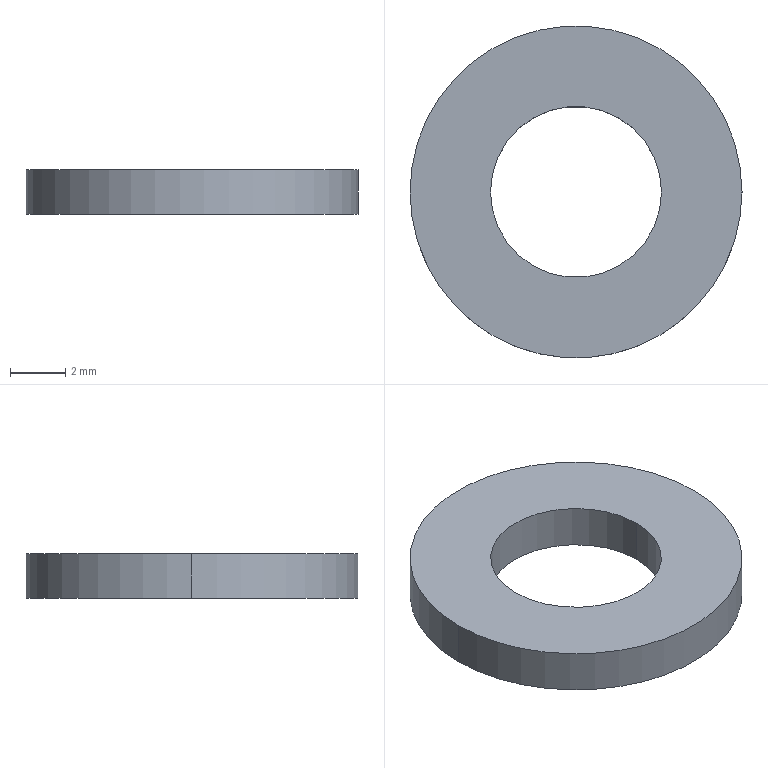Part | SolidWorks | features Extrusion 1 | 1 solid | 6 faces | box 12 x 12 x 1.6 mm | volume 132.962 mm3 | cylinder 4 | plane 2 | commonest cylinder face diameters 6.18 x2 12 x2
STEP:
#1=CARTESIAN_POINT('',(-3.09,0.,-1.6));
#2=VERTEX_POINT('',#1);
#3=CARTESIAN_POINT('',(3.09,0.,-1.6));
#4=VERTEX_POINT('',#3);
#5=CARTESIAN_POINT('',(0.,0.,-1.6));
#6=DIRECTION('',(0.,0.,1.));
#7=DIRECTION('',(1.,0.,0.));
#8=AXIS2_PLACEMENT_3D('',#5,#6,#7);
#9=CIRCLE('',#8,3.09);
#10=EDGE_CURVE('',#2,#4,#9,.T.);
#11=ORIENTED_EDGE('',*,*,#10,.F.);
#12=CARTESIAN_POINT('',(-3.09,0.,0.));
#13=VERTEX_POINT('',#12);
#14=CARTESIAN_POINT('',(-3.09,0.,-1.6));
#15=DIRECTION('',(0.,0.,1.));
#16=VECTOR('',#15,1000.);
#17=LINE('',#14,#16);
#18=EDGE_CURVE('',#2,#13,#17,.T.);
#19=ORIENTED_EDGE('',*,*,#18,.T.);
#20=CARTESIAN_POINT('',(3.09,0.,0.));
#21=VERTEX_POINT('',#20);
#22=CARTESIAN_POINT('',(0.,0.,0.));
#23=DIRECTION('',(0.,0.,1.));
#24=DIRECTION('',(1.,0.,0.));
#25=AXIS2_PLACEMENT_3D('',#22,#23,#24);
#26=CIRCLE('',#25,3.09);
#27=EDGE_CURVE('',#13,#21,#26,.T.);
#28=ORIENTED_EDGE('',*,*,#27,.T.);
#29=CARTESIAN_POINT('',(3.09,0.,-1.6));
#30=DIRECTION('',(0.,0.,1.));
#31=VECTOR('',#30,1000.);
#32=LINE('',#29,#31);
#33=EDGE_CURVE('',#4,#21,#32,.T.);
#34=ORIENTED_EDGE('',*,*,#33,.F.);
#35=EDGE_LOOP('',(#11,#19,#28,#34));
#36=FACE_OUTER_BOUND('',#35,.T.);
#37=CARTESIAN_POINT('',(0.,0.,-1.6));
#38=DIRECTION('',(0.,0.,1.));
#39=DIRECTION('',(1.,0.,0.));
#40=AXIS2_PLACEMENT_3D('',#37,#38,#39);
#41=CYLINDRICAL_SURFACE('',#40,3.09);
#42=ADVANCED_FACE('',(#36),#41,.F.);
#43=CARTESIAN_POINT('',(6.,0.,-1.6));
#44=VERTEX_POINT('',#43);
#45=CARTESIAN_POINT('',(-6.,0.,-1.6));
#46=VERTEX_POINT('',#45);
#47=CARTESIAN_POINT('',(0.,0.,-1.6));
#48=DIRECTION('',(0.,0.,1.));
#49=DIRECTION('',(1.,0.,0.));
#50=AXIS2_PLACEMENT_3D('',#47,#48,#49);
#51=CIRCLE('',#50,6.);
#52=EDGE_CURVE('',#44,#46,#51,.T.);
#53=ORIENTED_EDGE('',*,*,#52,.T.);
#54=CARTESIAN_POINT('',(-6.,0.,0.));
#55=VERTEX_POINT('',#54);
#56=CARTESIAN_POINT('',(-6.,0.,-1.6));
#57=DIRECTION('',(0.,0.,1.));
#58=VECTOR('',#57,1000.);
#59=LINE('',#56,#58);
#60=EDGE_CURVE('',#46,#55,#59,.T.);
#61=ORIENTED_EDGE('',*,*,#60,.T.);
#62=CARTESIAN_POINT('',(6.,0.,0.));
#63=VERTEX_POINT('',#62);
#64=CARTESIAN_POINT('',(0.,0.,0.));
#65=DIRECTION('',(0.,0.,1.));
#66=DIRECTION('',(1.,0.,0.));
#67=AXIS2_PLACEMENT_3D('',#64,#65,#66);
#68=CIRCLE('',#67,6.);
#69=EDGE_CURVE('',#63,#55,#68,.T.);
#70=ORIENTED_EDGE('',*,*,#69,.F.);
#71=CARTESIAN_POINT('',(6.,0.,-1.6));
#72=DIRECTION('',(0.,0.,1.));
#73=VECTOR('',#72,1000.);
#74=LINE('',#71,#73);
#75=EDGE_CURVE('',#44,#63,#74,.T.);
#76=ORIENTED_EDGE('',*,*,#75,.F.);
#77=EDGE_LOOP('',(#53,#61,#70,#76));
#78=FACE_OUTER_BOUND('',#77,.T.);
#79=CARTESIAN_POINT('',(0.,0.,-1.6));
#80=DIRECTION('',(0.,0.,1.));
#81=DIRECTION('',(1.,0.,0.));
#82=AXIS2_PLACEMENT_3D('',#79,#80,#81);
#83=CYLINDRICAL_SURFACE('',#82,6.);
#84=ADVANCED_FACE('',(#78),#83,.T.);
#85=ORIENTED_EDGE('',*,*,#60,.F.);
#86=CARTESIAN_POINT('',(0.,0.,-1.6));
#87=DIRECTION('',(0.,0.,1.));
#88=DIRECTION('',(1.,0.,0.));
#89=AXIS2_PLACEMENT_3D('',#86,#87,#88);
#90=CIRCLE('',#89,6.);
#91=EDGE_CURVE('',#46,#44,#90,.T.);
#92=ORIENTED_EDGE('',*,*,#91,.T.);
#93=ORIENTED_EDGE('',*,*,#75,.T.);
#94=CARTESIAN_POINT('',(0.,0.,0.));
#95=DIRECTION('',(0.,0.,1.));
#96=DIRECTION('',(1.,0.,0.));
#97=AXIS2_PLACEMENT_3D('',#94,#95,#96);
#98=CIRCLE('',#97,6.);
#99=EDGE_CURVE('',#55,#63,#98,.T.);
#100=ORIENTED_EDGE('',*,*,#99,.F.);
#101=EDGE_LOOP('',(#85,#92,#93,#100));
#102=FACE_OUTER_BOUND('',#101,.T.);
#103=CARTESIAN_POINT('',(0.,0.,-1.6));
#104=DIRECTION('',(0.,0.,1.));
#105=DIRECTION('',(1.,0.,0.));
#106=AXIS2_PLACEMENT_3D('',#103,#104,#105);
#107=CYLINDRICAL_SURFACE('',#106,6.);
#108=ADVANCED_FACE('',(#102),#107,.T.);
#109=CARTESIAN_POINT('',(0.,0.,-1.6));
#110=DIRECTION('',(0.,0.,1.));
#111=DIRECTION('',(1.,0.,0.));
#112=AXIS2_PLACEMENT_3D('',#109,#110,#111);
#113=CIRCLE('',#112,3.09);
#114=EDGE_CURVE('',#4,#2,#113,.T.);
#115=ORIENTED_EDGE('',*,*,#114,.T.);
#116=ORIENTED_EDGE('',*,*,#10,.T.);
#117=EDGE_LOOP('',(#115,#116));
#118=FACE_BOUND('',#117,.T.);
#119=ORIENTED_EDGE('',*,*,#52,.F.);
#120=ORIENTED_EDGE('',*,*,#91,.F.);
#121=EDGE_LOOP('',(#119,#120));
#122=FACE_OUTER_BOUND('',#121,.T.);
#123=CARTESIAN_POINT('',(0.,0.,-1.6));
#124=DIRECTION('',(0.,0.,1.));
#125=DIRECTION('',(1.,0.,0.));
#126=AXIS2_PLACEMENT_3D('',#123,#124,#125);
#127=PLANE('',#126);
#128=ADVANCED_FACE('',(#118,#122),#127,.F.);
#129=CARTESIAN_POINT('',(0.,0.,0.));
#130=DIRECTION('',(0.,0.,1.));
#131=DIRECTION('',(1.,0.,0.));
#132=AXIS2_PLACEMENT_3D('',#129,#130,#131);
#133=CIRCLE('',#132,3.09);
#134=EDGE_CURVE('',#21,#13,#133,.T.);
#135=ORIENTED_EDGE('',*,*,#134,.F.);
#136=ORIENTED_EDGE('',*,*,#27,.F.);
#137=EDGE_LOOP('',(#135,#136));
#138=FACE_BOUND('',#137,.T.);
#139=ORIENTED_EDGE('',*,*,#69,.T.);
#140=ORIENTED_EDGE('',*,*,#99,.T.);
#141=EDGE_LOOP('',(#139,#140));
#142=FACE_OUTER_BOUND('',#141,.T.);
#143=CARTESIAN_POINT('',(0.,0.,0.));
#144=DIRECTION('',(0.,0.,1.));
#145=DIRECTION('',(1.,0.,0.));
#146=AXIS2_PLACEMENT_3D('',#143,#144,#145);
#147=PLANE('',#146);
#148=ADVANCED_FACE('',(#138,#142),#147,.T.);
#149=ORIENTED_EDGE('',*,*,#18,.F.);
#150=ORIENTED_EDGE('',*,*,#114,.F.);
#151=ORIENTED_EDGE('',*,*,#33,.T.);
#152=ORIENTED_EDGE('',*,*,#134,.T.);
#153=EDGE_LOOP('',(#149,#150,#151,#152));
#154=FACE_OUTER_BOUND('',#153,.T.);
#155=CARTESIAN_POINT('',(0.,0.,-1.6));
#156=DIRECTION('',(0.,0.,1.));
#157=DIRECTION('',(1.,0.,0.));
#158=AXIS2_PLACEMENT_3D('',#155,#156,#157);
#159=CYLINDRICAL_SURFACE('',#158,3.09);
#160=ADVANCED_FACE('',(#154),#159,.F.);
#161=CLOSED_SHELL('',(#42,#84,#108,#128,#148,#160));
#162=MANIFOLD_SOLID_BREP('',#161);
#163=CARTESIAN_POINT('',(0.,0.,0.));
#164=DIRECTION('',(0.,0.,1.));
#165=DIRECTION('',(1.,0.,0.));
#166=AXIS2_PLACEMENT_3D('',#163,#164,#165);
#167=(LENGTH_UNIT()NAMED_UNIT(*)SI_UNIT(.MILLI.,.METRE.));
#168=UNCERTAINTY_MEASURE_WITH_UNIT(LENGTH_MEASURE(0.00001),#167,'','');
#169=(NAMED_UNIT(*)PLANE_ANGLE_UNIT()SI_UNIT($,.RADIAN.));
#170=(NAMED_UNIT(*)SI_UNIT($,.STERADIAN.)SOLID_ANGLE_UNIT());
#171=(GEOMETRIC_REPRESENTATION_CONTEXT(3)GLOBAL_UNCERTAINTY_ASSIGNED_CONTEXT((#168))GLOBAL_UNIT_ASSIGNED_CONTEXT((#167,#169,#170))REPRESENTATION_CONTEXT('',''));
#172=ADVANCED_BREP_SHAPE_REPRESENTATION('',(#162,#166),#171);